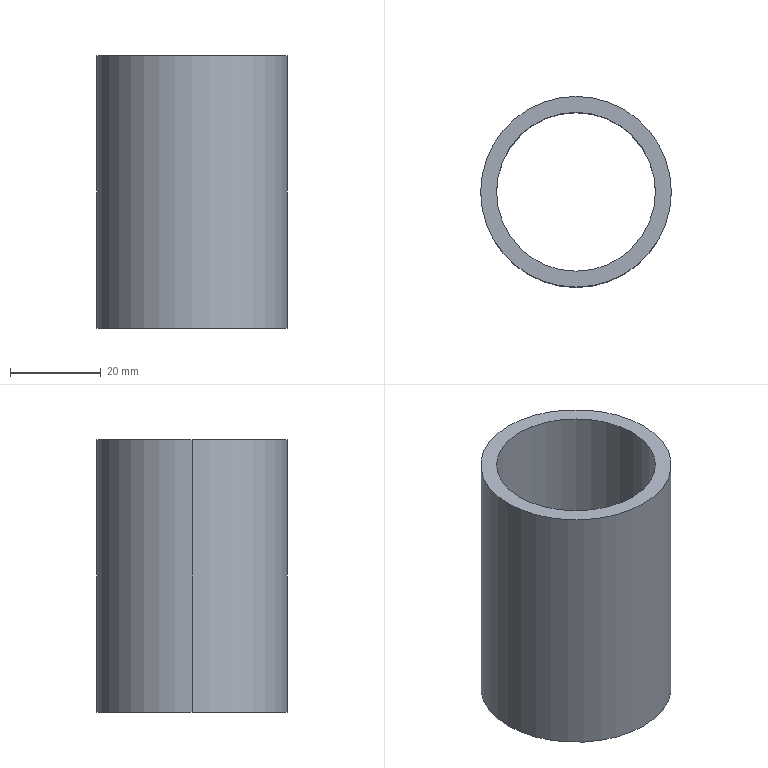Part | STEP file | 05-Spacer 3 | 1 solid | 6 faces | box 42 x 42 x 60 mm | volume 25400 mm3 | cylinder 4 | plane 2 | commonest cylinder face diameters 35 x2 42 x2
STEP:
#1=CARTESIAN_POINT('',(0.,0.,0.));
#2=DIRECTION('',(0.,0.,1.));
#3=DIRECTION('',(1.,0.,0.));
#4=AXIS2_PLACEMENT_3D('',#1,#2,#3);
#5=CARTESIAN_POINT('',(-17.5,0.,60.));
#6=VERTEX_POINT('',#5);
#7=CARTESIAN_POINT('',(-17.5,0.,0.));
#8=VERTEX_POINT('',#7);
#9=CARTESIAN_POINT('',(-17.5,0.,60.));
#10=DIRECTION('',(0.,0.,-1.));
#11=VECTOR('',#10,1.);
#12=LINE('',#9,#11);
#13=CARTESIAN_POINT('',(0.,0.,60.));
#14=DIRECTION('',(0.,0.,-1.));
#15=DIRECTION('',(-1.,0.,0.));
#16=AXIS2_PLACEMENT_3D('',#13,#14,#15);
#17=CYLINDRICAL_SURFACE('',#16,17.5);
#18=CARTESIAN_POINT('',(6.283,0.));
#19=DIRECTION('',(0.,1.));
#20=VECTOR('',#19,1.);
#21=LINE('',#18,#20);
#22=(GEOMETRIC_REPRESENTATION_CONTEXT(2)PARAMETRIC_REPRESENTATION_CONTEXT()REPRESENTATION_CONTEXT('',''));
#23=DEFINITIONAL_REPRESENTATION('',(#21),#22);
#24=PCURVE('',#17,#23);
#25=CARTESIAN_POINT('',(0.,0.,60.));
#26=DIRECTION('',(0.,0.,-1.));
#27=DIRECTION('',(-1.,0.,0.));
#28=AXIS2_PLACEMENT_3D('',#25,#26,#27);
#29=CYLINDRICAL_SURFACE('',#28,17.5);
#30=CARTESIAN_POINT('',(0.,0.));
#31=DIRECTION('',(0.,1.));
#32=VECTOR('',#31,1.);
#33=LINE('',#30,#32);
#34=(GEOMETRIC_REPRESENTATION_CONTEXT(2)PARAMETRIC_REPRESENTATION_CONTEXT()REPRESENTATION_CONTEXT('',''));
#35=DEFINITIONAL_REPRESENTATION('',(#33),#34);
#36=PCURVE('',#29,#35);
#37=SURFACE_CURVE('',#12,(#24,#36),.PCURVE_S1.);
#38=EDGE_CURVE('',#6,#8,#37,.T.);
#39=ORIENTED_EDGE('',*,*,#38,.T.);
#40=CARTESIAN_POINT('',(17.5,0.,0.));
#41=VERTEX_POINT('',#40);
#42=CARTESIAN_POINT('',(0.,0.,0.));
#43=DIRECTION('',(0.,0.,1.));
#44=DIRECTION('',(1.,0.,0.));
#45=AXIS2_PLACEMENT_3D('',#42,#43,#44);
#46=CIRCLE('',#45,17.5);
#47=CARTESIAN_POINT('',(9.425,60.));
#48=DIRECTION('',(-1.,0.));
#49=VECTOR('',#48,1.);
#50=LINE('',#47,#49);
#51=(GEOMETRIC_REPRESENTATION_CONTEXT(2)PARAMETRIC_REPRESENTATION_CONTEXT()REPRESENTATION_CONTEXT('',''));
#52=DEFINITIONAL_REPRESENTATION('',(#50),#51);
#53=PCURVE('',#17,#52);
#54=CARTESIAN_POINT('',(0.,0.,0.));
#55=DIRECTION('',(0.,0.,1.));
#56=DIRECTION('',(1.,0.,0.));
#57=AXIS2_PLACEMENT_3D('',#54,#55,#56);
#58=PLANE('',#57);
#59=CARTESIAN_POINT('',(0.,0.));
#60=DIRECTION('',(1.,0.));
#61=AXIS2_PLACEMENT_2D('',#59,#60);
#62=CIRCLE('',#61,17.5);
#63=(GEOMETRIC_REPRESENTATION_CONTEXT(2)PARAMETRIC_REPRESENTATION_CONTEXT()REPRESENTATION_CONTEXT('',''));
#64=DEFINITIONAL_REPRESENTATION('',(#62),#63);
#65=PCURVE('',#58,#64);
#66=SURFACE_CURVE('',#46,(#53,#65),.PCURVE_S1.);
#67=EDGE_CURVE('',#8,#41,#66,.T.);
#68=ORIENTED_EDGE('',*,*,#67,.T.);
#69=CARTESIAN_POINT('',(17.5,0.,60.));
#70=VERTEX_POINT('',#69);
#71=CARTESIAN_POINT('',(17.5,0.,60.));
#72=DIRECTION('',(0.,0.,-1.));
#73=VECTOR('',#72,1.);
#74=LINE('',#71,#73);
#75=CARTESIAN_POINT('',(3.142,0.));
#76=DIRECTION('',(0.,1.));
#77=VECTOR('',#76,1.);
#78=LINE('',#75,#77);
#79=(GEOMETRIC_REPRESENTATION_CONTEXT(2)PARAMETRIC_REPRESENTATION_CONTEXT()REPRESENTATION_CONTEXT('',''));
#80=DEFINITIONAL_REPRESENTATION('',(#78),#79);
#81=PCURVE('',#17,#80);
#82=CARTESIAN_POINT('',(3.142,0.));
#83=DIRECTION('',(0.,1.));
#84=VECTOR('',#83,1.);
#85=LINE('',#82,#84);
#86=(GEOMETRIC_REPRESENTATION_CONTEXT(2)PARAMETRIC_REPRESENTATION_CONTEXT()REPRESENTATION_CONTEXT('',''));
#87=DEFINITIONAL_REPRESENTATION('',(#85),#86);
#88=PCURVE('',#29,#87);
#89=SURFACE_CURVE('',#74,(#81,#88),.PCURVE_S1.);
#90=EDGE_CURVE('',#70,#41,#89,.T.);
#91=ORIENTED_EDGE('',*,*,#90,.F.);
#92=CARTESIAN_POINT('',(0.,0.,60.));
#93=DIRECTION('',(0.,0.,1.));
#94=DIRECTION('',(1.,0.,0.));
#95=AXIS2_PLACEMENT_3D('',#92,#93,#94);
#96=CIRCLE('',#95,17.5);
#97=CARTESIAN_POINT('',(9.425,0.));
#98=DIRECTION('',(-1.,0.));
#99=VECTOR('',#98,1.);
#100=LINE('',#97,#99);
#101=(GEOMETRIC_REPRESENTATION_CONTEXT(2)PARAMETRIC_REPRESENTATION_CONTEXT()REPRESENTATION_CONTEXT('',''));
#102=DEFINITIONAL_REPRESENTATION('',(#100),#101);
#103=PCURVE('',#17,#102);
#104=CARTESIAN_POINT('',(0.,0.,60.));
#105=DIRECTION('',(0.,0.,1.));
#106=DIRECTION('',(1.,0.,0.));
#107=AXIS2_PLACEMENT_3D('',#104,#105,#106);
#108=PLANE('',#107);
#109=CARTESIAN_POINT('',(0.,0.));
#110=DIRECTION('',(1.,0.));
#111=AXIS2_PLACEMENT_2D('',#109,#110);
#112=CIRCLE('',#111,17.5);
#113=(GEOMETRIC_REPRESENTATION_CONTEXT(2)PARAMETRIC_REPRESENTATION_CONTEXT()REPRESENTATION_CONTEXT('',''));
#114=DEFINITIONAL_REPRESENTATION('',(#112),#113);
#115=PCURVE('',#108,#114);
#116=SURFACE_CURVE('',#96,(#103,#115),.PCURVE_S1.);
#117=EDGE_CURVE('',#6,#70,#116,.T.);
#118=ORIENTED_EDGE('',*,*,#117,.F.);
#119=EDGE_LOOP('',(#39,#68,#91,#118));
#120=FACE_BOUND('',#119,.F.);
#121=ADVANCED_FACE('',(#120),#17,.F.);
#122=CARTESIAN_POINT('',(21.,0.,60.));
#123=VERTEX_POINT('',#122);
#124=CARTESIAN_POINT('',(-21.,0.,60.));
#125=VERTEX_POINT('',#124);
#126=CARTESIAN_POINT('',(0.,0.,60.));
#127=DIRECTION('',(0.,0.,1.));
#128=DIRECTION('',(1.,0.,0.));
#129=AXIS2_PLACEMENT_3D('',#126,#127,#128);
#130=CIRCLE('',#129,21.);
#131=CARTESIAN_POINT('',(0.,0.,60.));
#132=DIRECTION('',(0.,0.,-1.));
#133=DIRECTION('',(-1.,0.,0.));
#134=AXIS2_PLACEMENT_3D('',#131,#132,#133);
#135=CYLINDRICAL_SURFACE('',#134,21.);
#136=CARTESIAN_POINT('',(3.142,0.));
#137=DIRECTION('',(-1.,0.));
#138=VECTOR('',#137,1.);
#139=LINE('',#136,#138);
#140=(GEOMETRIC_REPRESENTATION_CONTEXT(2)PARAMETRIC_REPRESENTATION_CONTEXT()REPRESENTATION_CONTEXT('',''));
#141=DEFINITIONAL_REPRESENTATION('',(#139),#140);
#142=PCURVE('',#135,#141);
#143=CARTESIAN_POINT('',(0.,0.));
#144=DIRECTION('',(1.,0.));
#145=AXIS2_PLACEMENT_2D('',#143,#144);
#146=CIRCLE('',#145,21.);
#147=(GEOMETRIC_REPRESENTATION_CONTEXT(2)PARAMETRIC_REPRESENTATION_CONTEXT()REPRESENTATION_CONTEXT('',''));
#148=DEFINITIONAL_REPRESENTATION('',(#146),#147);
#149=PCURVE('',#108,#148);
#150=SURFACE_CURVE('',#130,(#142,#149),.PCURVE_S1.);
#151=EDGE_CURVE('',#123,#125,#150,.T.);
#152=ORIENTED_EDGE('',*,*,#151,.F.);
#153=CARTESIAN_POINT('',(21.,0.,0.));
#154=VERTEX_POINT('',#153);
#155=CARTESIAN_POINT('',(21.,0.,60.));
#156=DIRECTION('',(0.,0.,-1.));
#157=VECTOR('',#156,1.);
#158=LINE('',#155,#157);
#159=CARTESIAN_POINT('',(3.142,0.));
#160=DIRECTION('',(0.,1.));
#161=VECTOR('',#160,1.);
#162=LINE('',#159,#161);
#163=(GEOMETRIC_REPRESENTATION_CONTEXT(2)PARAMETRIC_REPRESENTATION_CONTEXT()REPRESENTATION_CONTEXT('',''));
#164=DEFINITIONAL_REPRESENTATION('',(#162),#163);
#165=PCURVE('',#135,#164);
#166=CARTESIAN_POINT('',(0.,0.,60.));
#167=DIRECTION('',(0.,0.,-1.));
#168=DIRECTION('',(-1.,0.,0.));
#169=AXIS2_PLACEMENT_3D('',#166,#167,#168);
#170=CYLINDRICAL_SURFACE('',#169,21.);
#171=CARTESIAN_POINT('',(3.142,0.));
#172=DIRECTION('',(0.,1.));
#173=VECTOR('',#172,1.);
#174=LINE('',#171,#173);
#175=(GEOMETRIC_REPRESENTATION_CONTEXT(2)PARAMETRIC_REPRESENTATION_CONTEXT()REPRESENTATION_CONTEXT('',''));
#176=DEFINITIONAL_REPRESENTATION('',(#174),#175);
#177=PCURVE('',#170,#176);
#178=SURFACE_CURVE('',#158,(#165,#177),.PCURVE_S1.);
#179=EDGE_CURVE('',#123,#154,#178,.T.);
#180=ORIENTED_EDGE('',*,*,#179,.T.);
#181=CARTESIAN_POINT('',(-21.,0.,0.));
#182=VERTEX_POINT('',#181);
#183=CARTESIAN_POINT('',(0.,0.,0.));
#184=DIRECTION('',(0.,0.,1.));
#185=DIRECTION('',(1.,0.,0.));
#186=AXIS2_PLACEMENT_3D('',#183,#184,#185);
#187=CIRCLE('',#186,21.);
#188=CARTESIAN_POINT('',(3.142,60.));
#189=DIRECTION('',(-1.,0.));
#190=VECTOR('',#189,1.);
#191=LINE('',#188,#190);
#192=(GEOMETRIC_REPRESENTATION_CONTEXT(2)PARAMETRIC_REPRESENTATION_CONTEXT()REPRESENTATION_CONTEXT('',''));
#193=DEFINITIONAL_REPRESENTATION('',(#191),#192);
#194=PCURVE('',#135,#193);
#195=CARTESIAN_POINT('',(0.,0.));
#196=DIRECTION('',(1.,0.));
#197=AXIS2_PLACEMENT_2D('',#195,#196);
#198=CIRCLE('',#197,21.);
#199=(GEOMETRIC_REPRESENTATION_CONTEXT(2)PARAMETRIC_REPRESENTATION_CONTEXT()REPRESENTATION_CONTEXT('',''));
#200=DEFINITIONAL_REPRESENTATION('',(#198),#199);
#201=PCURVE('',#58,#200);
#202=SURFACE_CURVE('',#187,(#194,#201),.PCURVE_S1.);
#203=EDGE_CURVE('',#154,#182,#202,.T.);
#204=ORIENTED_EDGE('',*,*,#203,.T.);
#205=CARTESIAN_POINT('',(-21.,0.,60.));
#206=DIRECTION('',(0.,0.,-1.));
#207=VECTOR('',#206,1.);
#208=LINE('',#205,#207);
#209=CARTESIAN_POINT('',(0.,0.));
#210=DIRECTION('',(0.,1.));
#211=VECTOR('',#210,1.);
#212=LINE('',#209,#211);
#213=(GEOMETRIC_REPRESENTATION_CONTEXT(2)PARAMETRIC_REPRESENTATION_CONTEXT()REPRESENTATION_CONTEXT('',''));
#214=DEFINITIONAL_REPRESENTATION('',(#212),#213);
#215=PCURVE('',#135,#214);
#216=CARTESIAN_POINT('',(6.283,0.));
#217=DIRECTION('',(0.,1.));
#218=VECTOR('',#217,1.);
#219=LINE('',#216,#218);
#220=(GEOMETRIC_REPRESENTATION_CONTEXT(2)PARAMETRIC_REPRESENTATION_CONTEXT()REPRESENTATION_CONTEXT('',''));
#221=DEFINITIONAL_REPRESENTATION('',(#219),#220);
#222=PCURVE('',#170,#221);
#223=SURFACE_CURVE('',#208,(#215,#222),.PCURVE_S1.);
#224=EDGE_CURVE('',#125,#182,#223,.T.);
#225=ORIENTED_EDGE('',*,*,#224,.F.);
#226=EDGE_LOOP('',(#152,#180,#204,#225));
#227=FACE_BOUND('',#226,.T.);
#228=ADVANCED_FACE('',(#227),#135,.T.);
#229=CARTESIAN_POINT('',(0.,0.,60.));
#230=DIRECTION('',(0.,0.,1.));
#231=DIRECTION('',(1.,0.,0.));
#232=AXIS2_PLACEMENT_3D('',#229,#230,#231);
#233=CIRCLE('',#232,21.);
#234=CARTESIAN_POINT('',(0.,0.));
#235=DIRECTION('',(1.,0.));
#236=AXIS2_PLACEMENT_2D('',#234,#235);
#237=CIRCLE('',#236,21.);
#238=(GEOMETRIC_REPRESENTATION_CONTEXT(2)PARAMETRIC_REPRESENTATION_CONTEXT()REPRESENTATION_CONTEXT('',''));
#239=DEFINITIONAL_REPRESENTATION('',(#237),#238);
#240=PCURVE('',#108,#239);
#241=CARTESIAN_POINT('',(9.425,0.));
#242=DIRECTION('',(-1.,0.));
#243=VECTOR('',#242,1.);
#244=LINE('',#241,#243);
#245=(GEOMETRIC_REPRESENTATION_CONTEXT(2)PARAMETRIC_REPRESENTATION_CONTEXT()REPRESENTATION_CONTEXT('',''));
#246=DEFINITIONAL_REPRESENTATION('',(#244),#245);
#247=PCURVE('',#170,#246);
#248=SURFACE_CURVE('',#233,(#240,#247),.PCURVE_S1.);
#249=EDGE_CURVE('',#125,#123,#248,.T.);
#250=ORIENTED_EDGE('',*,*,#249,.T.);
#251=ORIENTED_EDGE('',*,*,#151,.T.);
#252=EDGE_LOOP('',(#250,#251));
#253=FACE_BOUND('',#252,.T.);
#254=ORIENTED_EDGE('',*,*,#117,.F.);
#255=CARTESIAN_POINT('',(0.,0.,60.));
#256=DIRECTION('',(0.,0.,1.));
#257=DIRECTION('',(1.,0.,0.));
#258=AXIS2_PLACEMENT_3D('',#255,#256,#257);
#259=CIRCLE('',#258,17.5);
#260=CARTESIAN_POINT('',(0.,0.));
#261=DIRECTION('',(1.,0.));
#262=AXIS2_PLACEMENT_2D('',#260,#261);
#263=CIRCLE('',#262,17.5);
#264=(GEOMETRIC_REPRESENTATION_CONTEXT(2)PARAMETRIC_REPRESENTATION_CONTEXT()REPRESENTATION_CONTEXT('',''));
#265=DEFINITIONAL_REPRESENTATION('',(#263),#264);
#266=PCURVE('',#108,#265);
#267=CARTESIAN_POINT('',(3.142,0.));
#268=DIRECTION('',(-1.,0.));
#269=VECTOR('',#268,1.);
#270=LINE('',#267,#269);
#271=(GEOMETRIC_REPRESENTATION_CONTEXT(2)PARAMETRIC_REPRESENTATION_CONTEXT()REPRESENTATION_CONTEXT('',''));
#272=DEFINITIONAL_REPRESENTATION('',(#270),#271);
#273=PCURVE('',#29,#272);
#274=SURFACE_CURVE('',#259,(#266,#273),.PCURVE_S1.);
#275=EDGE_CURVE('',#70,#6,#274,.T.);
#276=ORIENTED_EDGE('',*,*,#275,.F.);
#277=EDGE_LOOP('',(#254,#276));
#278=FACE_BOUND('',#277,.T.);
#279=ADVANCED_FACE('',(#253,#278),#108,.T.);
#280=CARTESIAN_POINT('',(0.,0.,0.));
#281=DIRECTION('',(0.,0.,1.));
#282=DIRECTION('',(1.,0.,0.));
#283=AXIS2_PLACEMENT_3D('',#280,#281,#282);
#284=CIRCLE('',#283,21.);
#285=CARTESIAN_POINT('',(0.,0.));
#286=DIRECTION('',(1.,0.));
#287=AXIS2_PLACEMENT_2D('',#285,#286);
#288=CIRCLE('',#287,21.);
#289=(GEOMETRIC_REPRESENTATION_CONTEXT(2)PARAMETRIC_REPRESENTATION_CONTEXT()REPRESENTATION_CONTEXT('',''));
#290=DEFINITIONAL_REPRESENTATION('',(#288),#289);
#291=PCURVE('',#58,#290);
#292=CARTESIAN_POINT('',(9.425,60.));
#293=DIRECTION('',(-1.,0.));
#294=VECTOR('',#293,1.);
#295=LINE('',#292,#294);
#296=(GEOMETRIC_REPRESENTATION_CONTEXT(2)PARAMETRIC_REPRESENTATION_CONTEXT()REPRESENTATION_CONTEXT('',''));
#297=DEFINITIONAL_REPRESENTATION('',(#295),#296);
#298=PCURVE('',#170,#297);
#299=SURFACE_CURVE('',#284,(#291,#298),.PCURVE_S1.);
#300=EDGE_CURVE('',#182,#154,#299,.T.);
#301=ORIENTED_EDGE('',*,*,#300,.F.);
#302=ORIENTED_EDGE('',*,*,#203,.F.);
#303=EDGE_LOOP('',(#301,#302));
#304=FACE_BOUND('',#303,.T.);
#305=ORIENTED_EDGE('',*,*,#67,.T.);
#306=CARTESIAN_POINT('',(0.,0.,0.));
#307=DIRECTION('',(0.,0.,1.));
#308=DIRECTION('',(1.,0.,0.));
#309=AXIS2_PLACEMENT_3D('',#306,#307,#308);
#310=CIRCLE('',#309,17.5);
#311=CARTESIAN_POINT('',(0.,0.));
#312=DIRECTION('',(1.,0.));
#313=AXIS2_PLACEMENT_2D('',#311,#312);
#314=CIRCLE('',#313,17.5);
#315=(GEOMETRIC_REPRESENTATION_CONTEXT(2)PARAMETRIC_REPRESENTATION_CONTEXT()REPRESENTATION_CONTEXT('',''));
#316=DEFINITIONAL_REPRESENTATION('',(#314),#315);
#317=PCURVE('',#58,#316);
#318=CARTESIAN_POINT('',(3.142,60.));
#319=DIRECTION('',(-1.,0.));
#320=VECTOR('',#319,1.);
#321=LINE('',#318,#320);
#322=(GEOMETRIC_REPRESENTATION_CONTEXT(2)PARAMETRIC_REPRESENTATION_CONTEXT()REPRESENTATION_CONTEXT('',''));
#323=DEFINITIONAL_REPRESENTATION('',(#321),#322);
#324=PCURVE('',#29,#323);
#325=SURFACE_CURVE('',#310,(#317,#324),.PCURVE_S1.);
#326=EDGE_CURVE('',#41,#8,#325,.T.);
#327=ORIENTED_EDGE('',*,*,#326,.T.);
#328=EDGE_LOOP('',(#305,#327));
#329=FACE_BOUND('',#328,.T.);
#330=ADVANCED_FACE('',(#304,#329),#58,.F.);
#331=ORIENTED_EDGE('',*,*,#179,.F.);
#332=ORIENTED_EDGE('',*,*,#249,.F.);
#333=ORIENTED_EDGE('',*,*,#224,.T.);
#334=ORIENTED_EDGE('',*,*,#300,.T.);
#335=EDGE_LOOP('',(#331,#332,#333,#334));
#336=FACE_BOUND('',#335,.T.);
#337=ADVANCED_FACE('',(#336),#170,.T.);
#338=ORIENTED_EDGE('',*,*,#326,.T.);
#339=ORIENTED_EDGE('',*,*,#38,.F.);
#340=ORIENTED_EDGE('',*,*,#275,.F.);
#341=ORIENTED_EDGE('',*,*,#90,.T.);
#342=EDGE_LOOP('',(#338,#339,#340,#341));
#343=FACE_BOUND('',#342,.F.);
#344=ADVANCED_FACE('',(#343),#29,.F.);
#345=CLOSED_SHELL('',(#121,#228,#279,#330,#337,#344));
#346=MANIFOLD_SOLID_BREP('',#345);
#347=(LENGTH_UNIT()NAMED_UNIT(*)SI_UNIT(.MILLI.,.METRE.));
#348=UNCERTAINTY_MEASURE_WITH_UNIT(LENGTH_MEASURE(0.0000001),#347,'','');
#349=(NAMED_UNIT(*)PLANE_ANGLE_UNIT()SI_UNIT($,.RADIAN.));
#350=(NAMED_UNIT(*)SI_UNIT($,.STERADIAN.)SOLID_ANGLE_UNIT());
#351=(GEOMETRIC_REPRESENTATION_CONTEXT(3)GLOBAL_UNCERTAINTY_ASSIGNED_CONTEXT((#348))GLOBAL_UNIT_ASSIGNED_CONTEXT((#347,#349,#350))REPRESENTATION_CONTEXT('',''));
#352=ADVANCED_BREP_SHAPE_REPRESENTATION('',(#4,#346),#351);